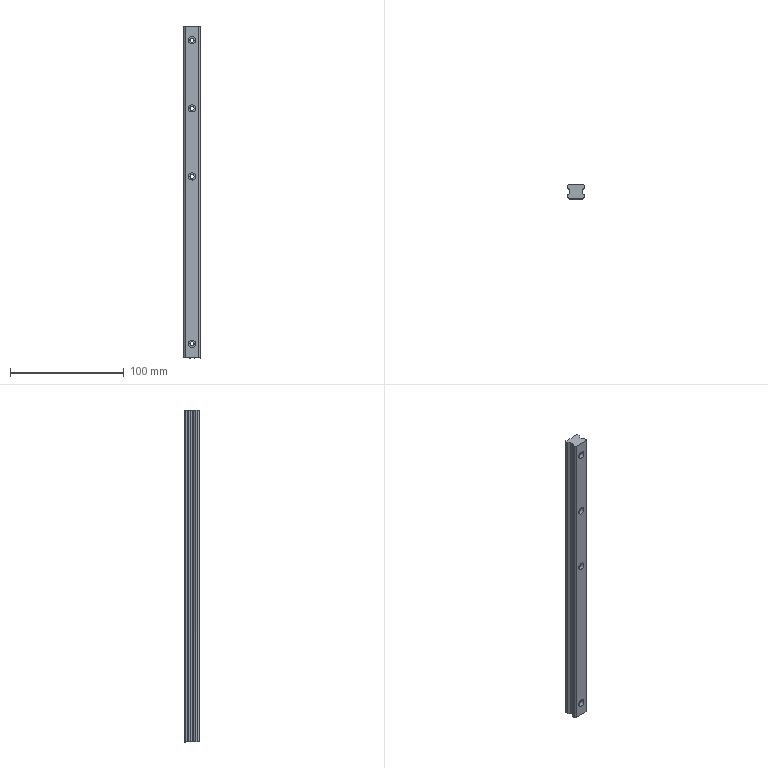Part | SolidWorks | features BaseBody 1 | 1 solid | 57 faces | box 15 x 12.5 x 292.5 mm | volume 46951 mm3 | cylinder 33 | plane 24 | commonest cylinder face diameters 0.6 x10 3.6 x8 6.5 x8 3 x5 1 x2